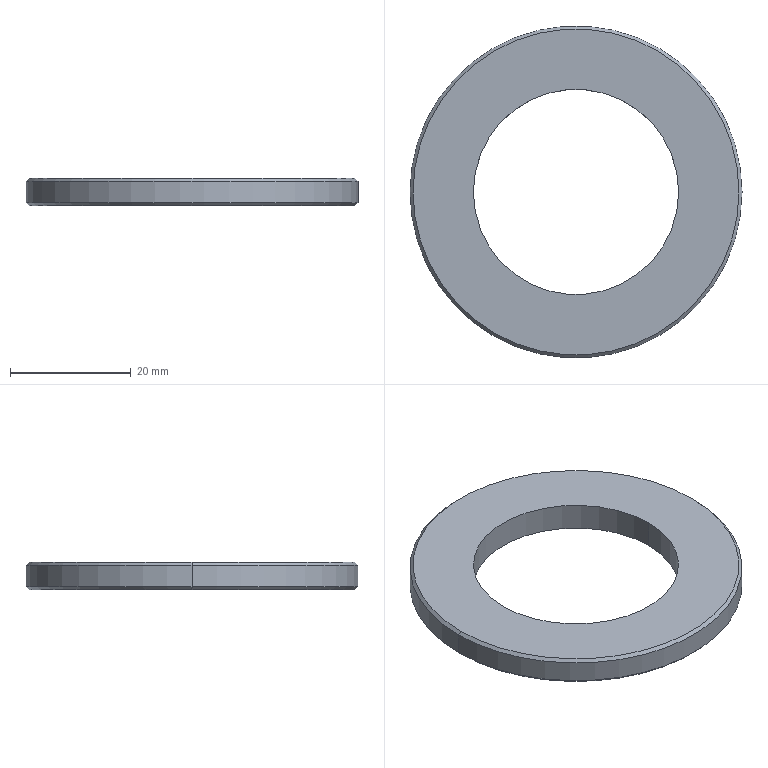Part | SolidWorks | features Chamfer 1, Extrusion 1 | 1 solid | 10 faces | box 55 x 55 x 4.6 mm | volume 6709 mm3 | cone 4 | cylinder 4 | plane 2 | commonest cylinder face diameters 34 x2 55 x2
STEP:
#1=CARTESIAN_POINT('',(27.,0.,4.6));
#2=VERTEX_POINT('',#1);
#3=CARTESIAN_POINT('',(-27.,0.,4.6));
#4=VERTEX_POINT('',#3);
#5=CARTESIAN_POINT('',(0.,0.,4.6));
#6=DIRECTION('',(0.,0.,1.));
#7=DIRECTION('',(1.,0.,0.));
#8=AXIS2_PLACEMENT_3D('',#5,#6,#7);
#9=CIRCLE('',#8,27.);
#10=EDGE_CURVE('',#2,#4,#9,.T.);
#11=ORIENTED_EDGE('',*,*,#10,.F.);
#12=CARTESIAN_POINT('',(27.5,0.,4.1));
#13=VERTEX_POINT('',#12);
#14=CARTESIAN_POINT('',(27.,0.,4.6));
#15=DIRECTION('',(0.7071,0.,-0.7071));
#16=VECTOR('',#15,1000.);
#17=LINE('',#14,#16);
#18=EDGE_CURVE('',#2,#13,#17,.T.);
#19=ORIENTED_EDGE('',*,*,#18,.T.);
#20=CARTESIAN_POINT('',(-27.5,0.,4.1));
#21=VERTEX_POINT('',#20);
#22=CARTESIAN_POINT('',(0.,0.,4.1));
#23=DIRECTION('',(0.,0.,-1.));
#24=DIRECTION('',(1.,0.,0.));
#25=AXIS2_PLACEMENT_3D('',#22,#23,#24);
#26=CIRCLE('',#25,27.5);
#27=EDGE_CURVE('',#21,#13,#26,.T.);
#28=ORIENTED_EDGE('',*,*,#27,.F.);
#29=CARTESIAN_POINT('',(-27.,0.,4.6));
#30=DIRECTION('',(-0.7071,0.,-0.7071));
#31=VECTOR('',#30,1000.);
#32=LINE('',#29,#31);
#33=EDGE_CURVE('',#4,#21,#32,.T.);
#34=ORIENTED_EDGE('',*,*,#33,.F.);
#35=EDGE_LOOP('',(#11,#19,#28,#34));
#36=FACE_OUTER_BOUND('',#35,.T.);
#37=CARTESIAN_POINT('',(0.,0.,4.6));
#38=DIRECTION('',(0.,0.,-1.));
#39=DIRECTION('',(-1.,0.,0.));
#40=AXIS2_PLACEMENT_3D('',#37,#38,#39);
#41=CONICAL_SURFACE('',#40,27.,0.7854);
#42=ADVANCED_FACE('',(#36),#41,.T.);
#43=CARTESIAN_POINT('',(-27.,0.,0.));
#44=VERTEX_POINT('',#43);
#45=CARTESIAN_POINT('',(27.,0.,0.));
#46=VERTEX_POINT('',#45);
#47=CARTESIAN_POINT('',(0.,0.,0.));
#48=DIRECTION('',(0.,0.,-1.));
#49=DIRECTION('',(1.,0.,0.));
#50=AXIS2_PLACEMENT_3D('',#47,#48,#49);
#51=CIRCLE('',#50,27.);
#52=EDGE_CURVE('',#44,#46,#51,.T.);
#53=ORIENTED_EDGE('',*,*,#52,.F.);
#54=CARTESIAN_POINT('',(-27.5,0.,0.5));
#55=VERTEX_POINT('',#54);
#56=CARTESIAN_POINT('',(-27.5,0.,0.5));
#57=DIRECTION('',(-0.7071,0.,0.7071));
#58=VECTOR('',#57,1000.);
#59=LINE('',#56,#58);
#60=EDGE_CURVE('',#44,#55,#59,.T.);
#61=ORIENTED_EDGE('',*,*,#60,.T.);
#62=CARTESIAN_POINT('',(27.5,0.,0.5));
#63=VERTEX_POINT('',#62);
#64=CARTESIAN_POINT('',(0.,0.,0.5));
#65=DIRECTION('',(0.,0.,1.));
#66=DIRECTION('',(1.,0.,0.));
#67=AXIS2_PLACEMENT_3D('',#64,#65,#66);
#68=CIRCLE('',#67,27.5);
#69=EDGE_CURVE('',#63,#55,#68,.T.);
#70=ORIENTED_EDGE('',*,*,#69,.F.);
#71=CARTESIAN_POINT('',(27.5,0.,0.5));
#72=DIRECTION('',(0.7071,0.,0.7071));
#73=VECTOR('',#72,1000.);
#74=LINE('',#71,#73);
#75=EDGE_CURVE('',#46,#63,#74,.T.);
#76=ORIENTED_EDGE('',*,*,#75,.F.);
#77=EDGE_LOOP('',(#53,#61,#70,#76));
#78=FACE_OUTER_BOUND('',#77,.T.);
#79=CARTESIAN_POINT('',(0.,0.,0.5));
#80=DIRECTION('',(0.,0.,1.));
#81=DIRECTION('',(1.,0.,0.));
#82=AXIS2_PLACEMENT_3D('',#79,#80,#81);
#83=CONICAL_SURFACE('',#82,27.5,0.7854);
#84=ADVANCED_FACE('',(#78),#83,.T.);
#85=CARTESIAN_POINT('',(-17.,0.,4.6));
#86=VERTEX_POINT('',#85);
#87=CARTESIAN_POINT('',(17.,0.,4.6));
#88=VERTEX_POINT('',#87);
#89=CARTESIAN_POINT('',(0.,0.,4.6));
#90=DIRECTION('',(0.,0.,1.));
#91=DIRECTION('',(1.,0.,0.));
#92=AXIS2_PLACEMENT_3D('',#89,#90,#91);
#93=CIRCLE('',#92,17.);
#94=EDGE_CURVE('',#86,#88,#93,.T.);
#95=ORIENTED_EDGE('',*,*,#94,.T.);
#96=CARTESIAN_POINT('',(17.,0.,0.));
#97=VERTEX_POINT('',#96);
#98=CARTESIAN_POINT('',(17.,0.,4.6));
#99=DIRECTION('',(0.,0.,-1.));
#100=VECTOR('',#99,1000.);
#101=LINE('',#98,#100);
#102=EDGE_CURVE('',#88,#97,#101,.T.);
#103=ORIENTED_EDGE('',*,*,#102,.T.);
#104=CARTESIAN_POINT('',(-17.,0.,0.));
#105=VERTEX_POINT('',#104);
#106=CARTESIAN_POINT('',(0.,0.,0.));
#107=DIRECTION('',(0.,0.,1.));
#108=DIRECTION('',(1.,0.,0.));
#109=AXIS2_PLACEMENT_3D('',#106,#107,#108);
#110=CIRCLE('',#109,17.);
#111=EDGE_CURVE('',#105,#97,#110,.T.);
#112=ORIENTED_EDGE('',*,*,#111,.F.);
#113=CARTESIAN_POINT('',(-17.,0.,4.6));
#114=DIRECTION('',(0.,0.,-1.));
#115=VECTOR('',#114,1000.);
#116=LINE('',#113,#115);
#117=EDGE_CURVE('',#86,#105,#116,.T.);
#118=ORIENTED_EDGE('',*,*,#117,.F.);
#119=EDGE_LOOP('',(#95,#103,#112,#118));
#120=FACE_OUTER_BOUND('',#119,.T.);
#121=CARTESIAN_POINT('',(0.,0.,4.6));
#122=DIRECTION('',(0.,0.,-1.));
#123=DIRECTION('',(-1.,0.,0.));
#124=AXIS2_PLACEMENT_3D('',#121,#122,#123);
#125=CYLINDRICAL_SURFACE('',#124,17.);
#126=ADVANCED_FACE('',(#120),#125,.F.);
#127=ORIENTED_EDGE('',*,*,#27,.T.);
#128=CARTESIAN_POINT('',(27.5,0.,4.6));
#129=DIRECTION('',(0.,0.,-1.));
#130=VECTOR('',#129,1000.);
#131=LINE('',#128,#130);
#132=EDGE_CURVE('',#13,#63,#131,.T.);
#133=ORIENTED_EDGE('',*,*,#132,.T.);
#134=ORIENTED_EDGE('',*,*,#69,.T.);
#135=CARTESIAN_POINT('',(-27.5,0.,4.6));
#136=DIRECTION('',(0.,0.,-1.));
#137=VECTOR('',#136,1000.);
#138=LINE('',#135,#137);
#139=EDGE_CURVE('',#21,#55,#138,.T.);
#140=ORIENTED_EDGE('',*,*,#139,.F.);
#141=EDGE_LOOP('',(#127,#133,#134,#140));
#142=FACE_OUTER_BOUND('',#141,.T.);
#143=CARTESIAN_POINT('',(0.,0.,4.6));
#144=DIRECTION('',(0.,0.,-1.));
#145=DIRECTION('',(-1.,0.,0.));
#146=AXIS2_PLACEMENT_3D('',#143,#144,#145);
#147=CYLINDRICAL_SURFACE('',#146,27.5);
#148=ADVANCED_FACE('',(#142),#147,.T.);
#149=CARTESIAN_POINT('',(0.,0.,4.6));
#150=DIRECTION('',(0.,0.,1.));
#151=DIRECTION('',(1.,0.,0.));
#152=AXIS2_PLACEMENT_3D('',#149,#150,#151);
#153=CIRCLE('',#152,27.);
#154=EDGE_CURVE('',#4,#2,#153,.T.);
#155=ORIENTED_EDGE('',*,*,#154,.T.);
#156=ORIENTED_EDGE('',*,*,#10,.T.);
#157=EDGE_LOOP('',(#155,#156));
#158=FACE_OUTER_BOUND('',#157,.T.);
#159=ORIENTED_EDGE('',*,*,#94,.F.);
#160=CARTESIAN_POINT('',(0.,0.,4.6));
#161=DIRECTION('',(0.,0.,1.));
#162=DIRECTION('',(1.,0.,0.));
#163=AXIS2_PLACEMENT_3D('',#160,#161,#162);
#164=CIRCLE('',#163,17.);
#165=EDGE_CURVE('',#88,#86,#164,.T.);
#166=ORIENTED_EDGE('',*,*,#165,.F.);
#167=EDGE_LOOP('',(#159,#166));
#168=FACE_BOUND('',#167,.T.);
#169=CARTESIAN_POINT('',(0.,0.,4.6));
#170=DIRECTION('',(0.,0.,1.));
#171=DIRECTION('',(1.,0.,0.));
#172=AXIS2_PLACEMENT_3D('',#169,#170,#171);
#173=PLANE('',#172);
#174=ADVANCED_FACE('',(#158,#168),#173,.T.);
#175=CARTESIAN_POINT('',(0.,0.,0.));
#176=DIRECTION('',(0.,0.,-1.));
#177=DIRECTION('',(1.,0.,0.));
#178=AXIS2_PLACEMENT_3D('',#175,#176,#177);
#179=CIRCLE('',#178,27.);
#180=EDGE_CURVE('',#46,#44,#179,.T.);
#181=ORIENTED_EDGE('',*,*,#180,.T.);
#182=ORIENTED_EDGE('',*,*,#52,.T.);
#183=EDGE_LOOP('',(#181,#182));
#184=FACE_OUTER_BOUND('',#183,.T.);
#185=ORIENTED_EDGE('',*,*,#111,.T.);
#186=CARTESIAN_POINT('',(0.,0.,0.));
#187=DIRECTION('',(0.,0.,1.));
#188=DIRECTION('',(1.,0.,0.));
#189=AXIS2_PLACEMENT_3D('',#186,#187,#188);
#190=CIRCLE('',#189,17.);
#191=EDGE_CURVE('',#97,#105,#190,.T.);
#192=ORIENTED_EDGE('',*,*,#191,.T.);
#193=EDGE_LOOP('',(#185,#192));
#194=FACE_BOUND('',#193,.T.);
#195=CARTESIAN_POINT('',(0.,0.,0.));
#196=DIRECTION('',(0.,0.,1.));
#197=DIRECTION('',(1.,0.,0.));
#198=AXIS2_PLACEMENT_3D('',#195,#196,#197);
#199=PLANE('',#198);
#200=ADVANCED_FACE('',(#184,#194),#199,.F.);
#201=ORIENTED_EDGE('',*,*,#132,.F.);
#202=CARTESIAN_POINT('',(0.,0.,4.1));
#203=DIRECTION('',(0.,0.,-1.));
#204=DIRECTION('',(1.,0.,0.));
#205=AXIS2_PLACEMENT_3D('',#202,#203,#204);
#206=CIRCLE('',#205,27.5);
#207=EDGE_CURVE('',#13,#21,#206,.T.);
#208=ORIENTED_EDGE('',*,*,#207,.T.);
#209=ORIENTED_EDGE('',*,*,#139,.T.);
#210=CARTESIAN_POINT('',(0.,0.,0.5));
#211=DIRECTION('',(0.,0.,1.));
#212=DIRECTION('',(1.,0.,0.));
#213=AXIS2_PLACEMENT_3D('',#210,#211,#212);
#214=CIRCLE('',#213,27.5);
#215=EDGE_CURVE('',#55,#63,#214,.T.);
#216=ORIENTED_EDGE('',*,*,#215,.T.);
#217=EDGE_LOOP('',(#201,#208,#209,#216));
#218=FACE_OUTER_BOUND('',#217,.T.);
#219=CARTESIAN_POINT('',(0.,0.,4.6));
#220=DIRECTION('',(0.,0.,-1.));
#221=DIRECTION('',(-1.,0.,0.));
#222=AXIS2_PLACEMENT_3D('',#219,#220,#221);
#223=CYLINDRICAL_SURFACE('',#222,27.5);
#224=ADVANCED_FACE('',(#218),#223,.T.);
#225=ORIENTED_EDGE('',*,*,#102,.F.);
#226=ORIENTED_EDGE('',*,*,#165,.T.);
#227=ORIENTED_EDGE('',*,*,#117,.T.);
#228=ORIENTED_EDGE('',*,*,#191,.F.);
#229=EDGE_LOOP('',(#225,#226,#227,#228));
#230=FACE_OUTER_BOUND('',#229,.T.);
#231=CARTESIAN_POINT('',(0.,0.,4.6));
#232=DIRECTION('',(0.,0.,-1.));
#233=DIRECTION('',(-1.,0.,0.));
#234=AXIS2_PLACEMENT_3D('',#231,#232,#233);
#235=CYLINDRICAL_SURFACE('',#234,17.);
#236=ADVANCED_FACE('',(#230),#235,.F.);
#237=ORIENTED_EDGE('',*,*,#60,.F.);
#238=ORIENTED_EDGE('',*,*,#180,.F.);
#239=ORIENTED_EDGE('',*,*,#75,.T.);
#240=ORIENTED_EDGE('',*,*,#215,.F.);
#241=EDGE_LOOP('',(#237,#238,#239,#240));
#242=FACE_OUTER_BOUND('',#241,.T.);
#243=CARTESIAN_POINT('',(0.,0.,0.5));
#244=DIRECTION('',(0.,0.,1.));
#245=DIRECTION('',(1.,0.,0.));
#246=AXIS2_PLACEMENT_3D('',#243,#244,#245);
#247=CONICAL_SURFACE('',#246,27.5,0.7854);
#248=ADVANCED_FACE('',(#242),#247,.T.);
#249=ORIENTED_EDGE('',*,*,#18,.F.);
#250=ORIENTED_EDGE('',*,*,#154,.F.);
#251=ORIENTED_EDGE('',*,*,#33,.T.);
#252=ORIENTED_EDGE('',*,*,#207,.F.);
#253=EDGE_LOOP('',(#249,#250,#251,#252));
#254=FACE_OUTER_BOUND('',#253,.T.);
#255=CARTESIAN_POINT('',(0.,0.,4.6));
#256=DIRECTION('',(0.,0.,-1.));
#257=DIRECTION('',(-1.,0.,0.));
#258=AXIS2_PLACEMENT_3D('',#255,#256,#257);
#259=CONICAL_SURFACE('',#258,27.,0.7854);
#260=ADVANCED_FACE('',(#254),#259,.T.);
#261=CLOSED_SHELL('',(#42,#84,#126,#148,#174,#200,#224,#236,#248,#260));
#262=MANIFOLD_SOLID_BREP('',#261);
#263=CARTESIAN_POINT('',(0.,0.,0.));
#264=DIRECTION('',(0.,0.,1.));
#265=DIRECTION('',(1.,0.,0.));
#266=AXIS2_PLACEMENT_3D('',#263,#264,#265);
#267=(LENGTH_UNIT()NAMED_UNIT(*)SI_UNIT(.MILLI.,.METRE.));
#268=UNCERTAINTY_MEASURE_WITH_UNIT(LENGTH_MEASURE(0.00001),#267,'','');
#269=(NAMED_UNIT(*)PLANE_ANGLE_UNIT()SI_UNIT($,.RADIAN.));
#270=(NAMED_UNIT(*)SI_UNIT($,.STERADIAN.)SOLID_ANGLE_UNIT());
#271=(GEOMETRIC_REPRESENTATION_CONTEXT(3)GLOBAL_UNCERTAINTY_ASSIGNED_CONTEXT((#268))GLOBAL_UNIT_ASSIGNED_CONTEXT((#267,#269,#270))REPRESENTATION_CONTEXT('',''));
#272=ADVANCED_BREP_SHAPE_REPRESENTATION('',(#262,#266),#271);